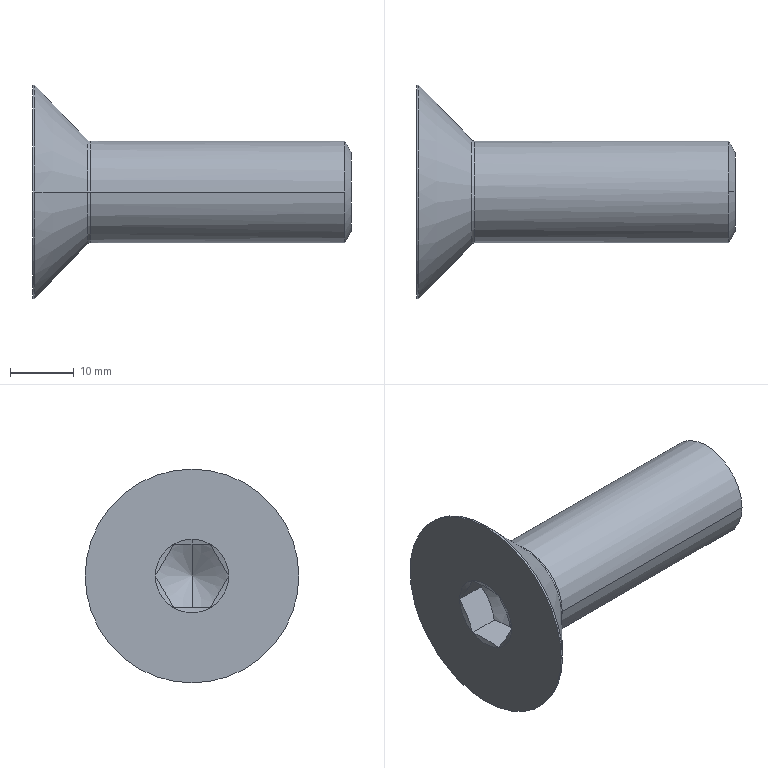Part | STEP file | GB/T 70.3-2000 hex socket countersunk screw M16×50 (8.8 grade) | 1 solid | 27 faces | box 50 x 33.6 x 33.6 mm | volume 12258 mm3 | cone 13 | plane 8 | cylinder 4 | torus 2 | commonest cylinder face diameters 16 x2 33.6 x2